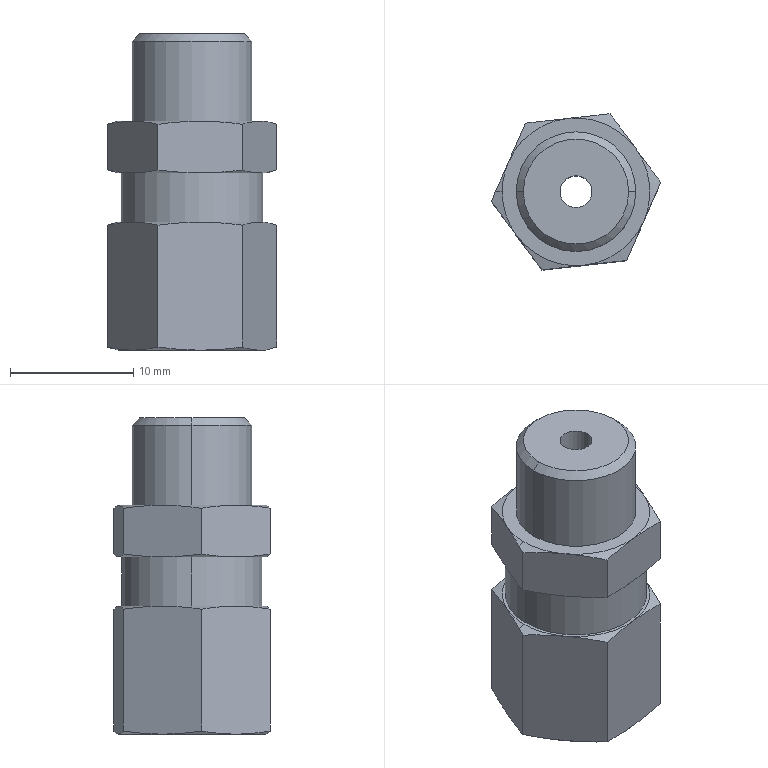Part | SolidWorks | features BaseBody 1 | 1 solid | 59 faces | box 13.769 x 12.7 x 25.7 mm | volume 2253 mm3 | cone 34 | plane 17 | cylinder 8 | commonest cylinder face diameters 2.6 x2 8.566 x2 9.728 x2 11.5 x2